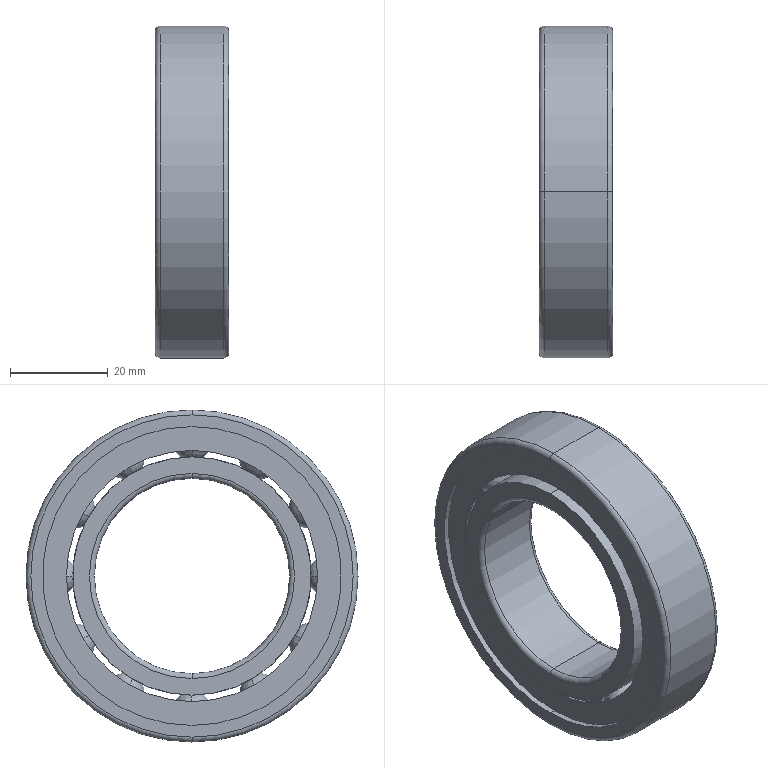Part | SolidWorks | 1 solid | 196 faces | box 15 x 68 x 68 mm | volume 23045 mm3 | sphere 96 | torus 44 | plane 32 | cylinder 24 | commonest cylinder face diameters 61.2 x8 48.8 x4 51.44 x4 40 x2 52.8 x2 57.2 x2